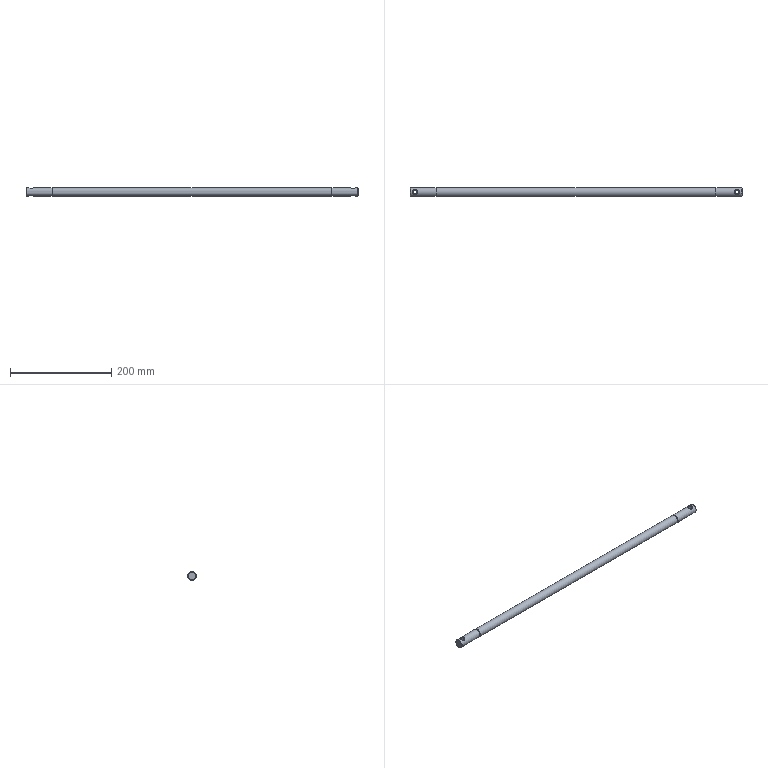Part | STEP file | Q7C0803 | 1 solid | 19 faces | box 655 x 17 x 17 mm | volume 147236 mm3 | cylinder 7 | plane 6 | spline 4 | cone 2 | commonest cylinder face diameters 17 x3 8 x2 15.6 x2